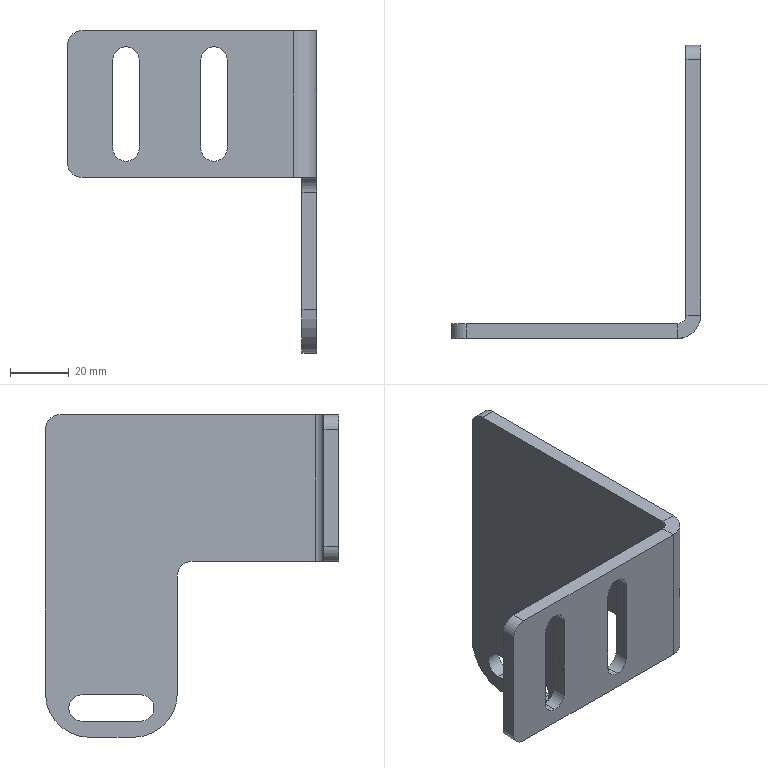Part | STEP file | 1 solid | 36 faces | box 85 x 100 x 110 mm | volume 52819 mm3 | plane 20 | cylinder 16 | commonest cylinder face diameters 9 x8 10 x4 30 x2 6 x1 16 x1